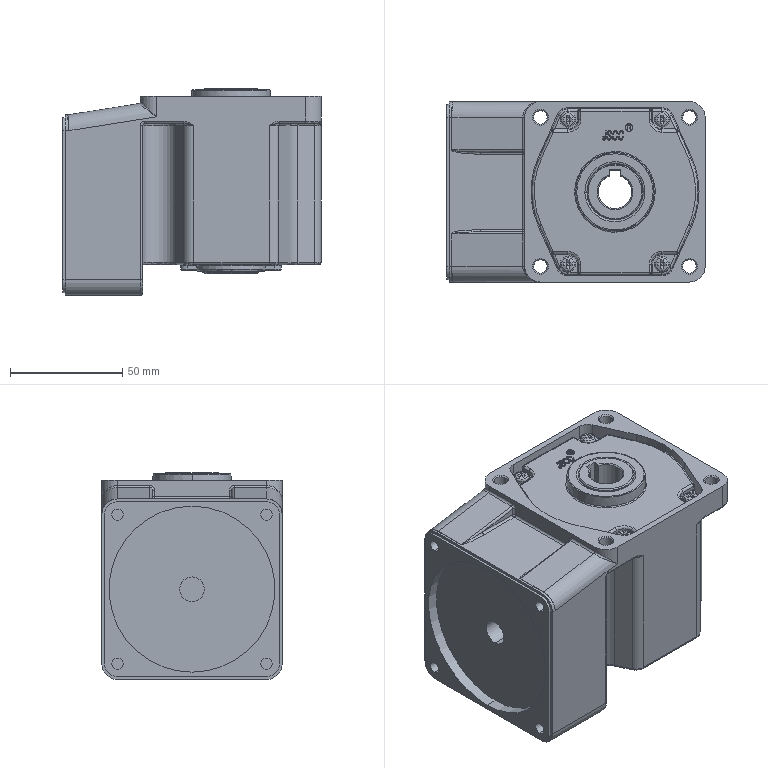Part | STEP file | 80GK-RC | 1 solid | 670 faces | box 115.25 x 80.5 x 92.25 mm | volume 602584 mm3 | plane 233 | cylinder 213 | spline 198 | cone 26 | commonest cylinder face diameters 2 x68 1 x16 6 x11 14 x11 15 x9 4 x8